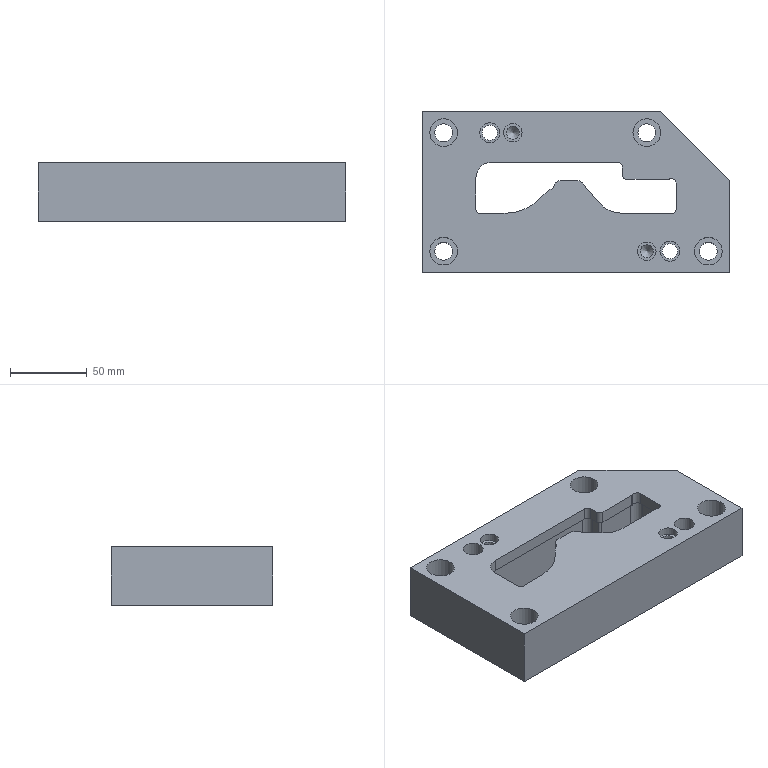Part | STEP file | lll_id210_x_t | 1 solid | 84 faces | box 200 x 105 x 38 mm | volume 586151 mm3 | cylinder 46 | plane 36 | cone 2 | commonest cylinder face diameters 6 x8 3 x4 9 x4 11.509 x4 18.008 x4 8 x3